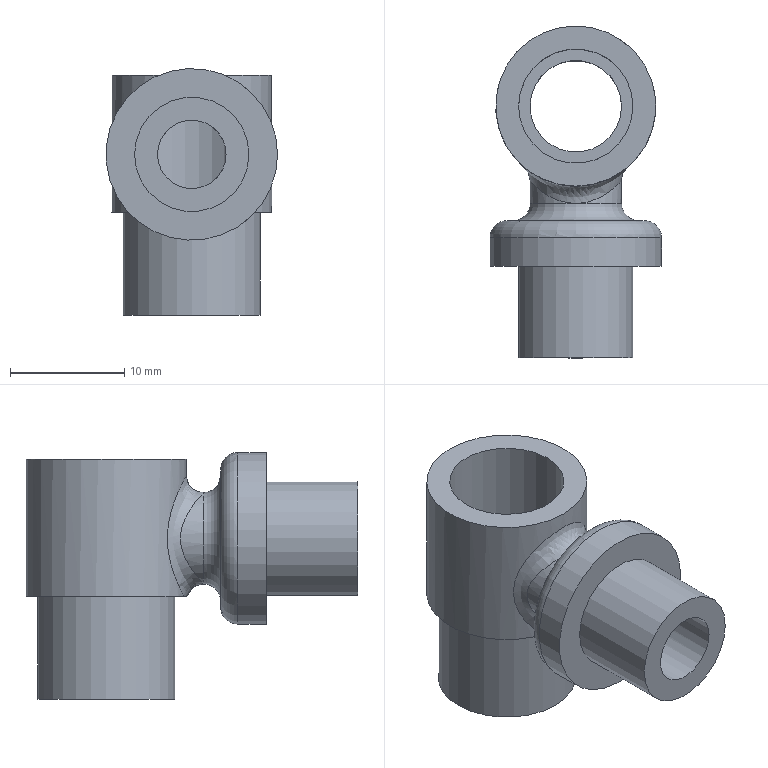Part | STEP file | 1-65.1 | 1 solid | 20 faces | box 15 x 29 x 21.57 mm | volume 2510 mm3 | cylinder 10 | plane 7 | torus 2 | spline 1 | commonest cylinder face diameters 8 x4 10 x2 6 x1 12 x1 14 x1 15 x1